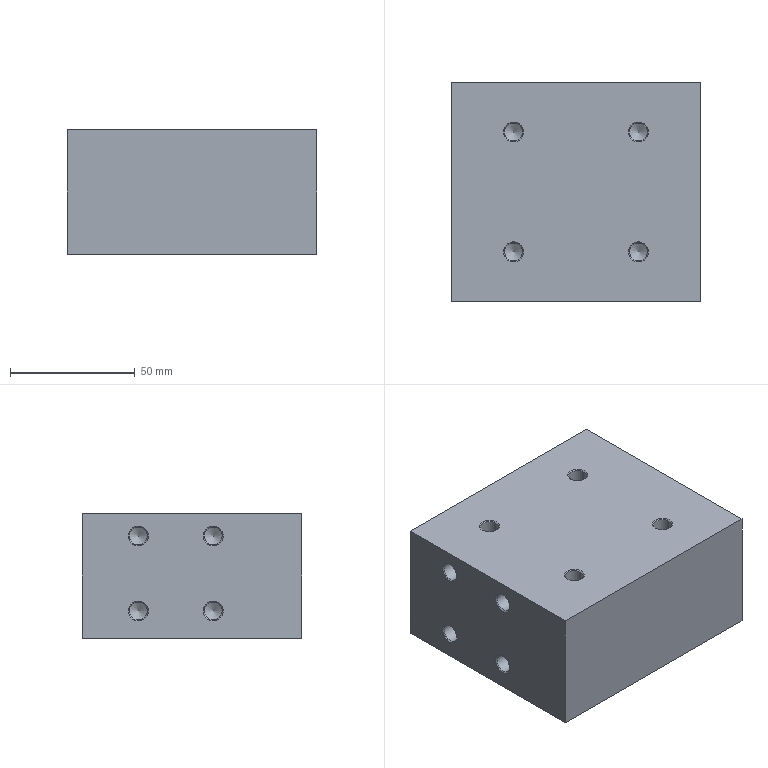Part | NX | features SIMPLE HOLE 8, SYMBOLIC_THREAD 8, DATUM_CSYS 4, SKETCH 3, HOLE PACKAGE 2, EXTRUDE 1 | 1 solid | 30 faces | box 100 x 88 x 50 mm | volume 433073 mm3 | cone 16 | cylinder 8 | plane 6 | commonest cylinder face diameters 7.2 x8
STEP:
#1=CARTESIAN_POINT('',(0.,69.5,41.));
#2=VERTEX_POINT('',#1);
#3=CARTESIAN_POINT('',(0.,65.5,41.));
#4=DIRECTION('',(1.,0.,0.));
#5=DIRECTION('',(0.,1.,0.));
#6=AXIS2_PLACEMENT_3D('',#3,#4,#5);
#7=CIRCLE('',#6,4.);
#8=EDGE_CURVE('',#2,#2,#7,.T.);
#9=ORIENTED_EDGE('',*,*,#8,.T.);
#10=EDGE_LOOP('',(#9));
#11=FACE_BOUND('',#10,.T.);
#12=CARTESIAN_POINT('',(0.,69.5,11.));
#13=VERTEX_POINT('',#12);
#14=CARTESIAN_POINT('',(0.,65.5,11.));
#15=DIRECTION('',(1.,0.,0.));
#16=DIRECTION('',(0.,1.,0.));
#17=AXIS2_PLACEMENT_3D('',#14,#15,#16);
#18=CIRCLE('',#17,4.);
#19=EDGE_CURVE('',#13,#13,#18,.T.);
#20=ORIENTED_EDGE('',*,*,#19,.T.);
#21=EDGE_LOOP('',(#20));
#22=FACE_BOUND('',#21,.T.);
#23=CARTESIAN_POINT('',(0.,39.5,41.));
#24=VERTEX_POINT('',#23);
#25=CARTESIAN_POINT('',(0.,35.5,41.));
#26=DIRECTION('',(1.,0.,0.));
#27=DIRECTION('',(0.,1.,0.));
#28=AXIS2_PLACEMENT_3D('',#25,#26,#27);
#29=CIRCLE('',#28,4.);
#30=EDGE_CURVE('',#24,#24,#29,.T.);
#31=ORIENTED_EDGE('',*,*,#30,.T.);
#32=EDGE_LOOP('',(#31));
#33=FACE_BOUND('',#32,.T.);
#34=CARTESIAN_POINT('',(0.,39.5,11.));
#35=VERTEX_POINT('',#34);
#36=CARTESIAN_POINT('',(0.,35.5,11.));
#37=DIRECTION('',(1.,0.,0.));
#38=DIRECTION('',(0.,1.,0.));
#39=AXIS2_PLACEMENT_3D('',#36,#37,#38);
#40=CIRCLE('',#39,4.);
#41=EDGE_CURVE('',#35,#35,#40,.T.);
#42=ORIENTED_EDGE('',*,*,#41,.T.);
#43=EDGE_LOOP('',(#42));
#44=FACE_BOUND('',#43,.T.);
#45=CARTESIAN_POINT('',(0.,88.,0.));
#46=VERTEX_POINT('',#45);
#47=CARTESIAN_POINT('',(0.,0.,0.));
#48=VERTEX_POINT('',#47);
#49=CARTESIAN_POINT('',(0.,88.,0.));
#50=DIRECTION('',(0.,-1.,0.));
#51=VECTOR('',#50,1000.);
#52=LINE('',#49,#51);
#53=EDGE_CURVE('',#46,#48,#52,.T.);
#54=ORIENTED_EDGE('',*,*,#53,.T.);
#55=CARTESIAN_POINT('',(0.,0.,50.));
#56=VERTEX_POINT('',#55);
#57=CARTESIAN_POINT('',(0.,0.,50.));
#58=DIRECTION('',(0.,0.,-1.));
#59=VECTOR('',#58,1000.);
#60=LINE('',#57,#59);
#61=EDGE_CURVE('',#56,#48,#60,.T.);
#62=ORIENTED_EDGE('',*,*,#61,.F.);
#63=CARTESIAN_POINT('',(0.,88.,50.));
#64=VERTEX_POINT('',#63);
#65=CARTESIAN_POINT('',(0.,88.,50.));
#66=DIRECTION('',(0.,-1.,0.));
#67=VECTOR('',#66,1000.);
#68=LINE('',#65,#67);
#69=EDGE_CURVE('',#64,#56,#68,.T.);
#70=ORIENTED_EDGE('',*,*,#69,.F.);
#71=CARTESIAN_POINT('',(0.,88.,50.));
#72=DIRECTION('',(0.,0.,-1.));
#73=VECTOR('',#72,1000.);
#74=LINE('',#71,#73);
#75=EDGE_CURVE('',#64,#46,#74,.T.);
#76=ORIENTED_EDGE('',*,*,#75,.T.);
#77=EDGE_LOOP('',(#54,#62,#70,#76));
#78=FACE_BOUND('',#77,.T.);
#79=CARTESIAN_POINT('',(0.,88.,50.));
#80=DIRECTION('',(1.,0.,0.));
#81=DIRECTION('',(0.,1.,0.));
#82=AXIS2_PLACEMENT_3D('',#79,#80,#81);
#83=PLANE('',#82);
#84=ADVANCED_FACE('',(#11,#22,#33,#44,#78),#83,.F.);
#85=CARTESIAN_POINT('',(100.,0.,0.));
#86=VERTEX_POINT('',#85);
#87=CARTESIAN_POINT('',(0.,0.,0.));
#88=DIRECTION('',(1.,0.,0.));
#89=VECTOR('',#88,1000.);
#90=LINE('',#87,#89);
#91=EDGE_CURVE('',#48,#86,#90,.T.);
#92=ORIENTED_EDGE('',*,*,#91,.T.);
#93=CARTESIAN_POINT('',(100.,0.,50.));
#94=VERTEX_POINT('',#93);
#95=CARTESIAN_POINT('',(100.,0.,50.));
#96=DIRECTION('',(0.,0.,-1.));
#97=VECTOR('',#96,1000.);
#98=LINE('',#95,#97);
#99=EDGE_CURVE('',#94,#86,#98,.T.);
#100=ORIENTED_EDGE('',*,*,#99,.F.);
#101=CARTESIAN_POINT('',(0.,0.,50.));
#102=DIRECTION('',(1.,0.,0.));
#103=VECTOR('',#102,1000.);
#104=LINE('',#101,#103);
#105=EDGE_CURVE('',#56,#94,#104,.T.);
#106=ORIENTED_EDGE('',*,*,#105,.F.);
#107=ORIENTED_EDGE('',*,*,#61,.T.);
#108=EDGE_LOOP('',(#92,#100,#106,#107));
#109=FACE_BOUND('',#108,.T.);
#110=CARTESIAN_POINT('',(0.,0.,50.));
#111=DIRECTION('',(0.,1.,0.));
#112=DIRECTION('',(0.,0.,1.));
#113=AXIS2_PLACEMENT_3D('',#110,#111,#112);
#114=PLANE('',#113);
#115=ADVANCED_FACE('',(#109),#114,.F.);
#116=CARTESIAN_POINT('',(100.,88.,0.));
#117=VERTEX_POINT('',#116);
#118=CARTESIAN_POINT('',(100.,0.,0.));
#119=DIRECTION('',(0.,1.,0.));
#120=VECTOR('',#119,1000.);
#121=LINE('',#118,#120);
#122=EDGE_CURVE('',#86,#117,#121,.T.);
#123=ORIENTED_EDGE('',*,*,#122,.T.);
#124=CARTESIAN_POINT('',(100.,88.,50.));
#125=VERTEX_POINT('',#124);
#126=CARTESIAN_POINT('',(100.,88.,50.));
#127=DIRECTION('',(0.,0.,-1.));
#128=VECTOR('',#127,1000.);
#129=LINE('',#126,#128);
#130=EDGE_CURVE('',#125,#117,#129,.T.);
#131=ORIENTED_EDGE('',*,*,#130,.F.);
#132=CARTESIAN_POINT('',(100.,0.,50.));
#133=DIRECTION('',(0.,1.,0.));
#134=VECTOR('',#133,1000.);
#135=LINE('',#132,#134);
#136=EDGE_CURVE('',#94,#125,#135,.T.);
#137=ORIENTED_EDGE('',*,*,#136,.F.);
#138=ORIENTED_EDGE('',*,*,#99,.T.);
#139=EDGE_LOOP('',(#123,#131,#137,#138));
#140=FACE_BOUND('',#139,.T.);
#141=CARTESIAN_POINT('',(100.,0.,50.));
#142=DIRECTION('',(-1.,0.,0.));
#143=DIRECTION('',(0.,-1.,0.));
#144=AXIS2_PLACEMENT_3D('',#141,#142,#143);
#145=PLANE('',#144);
#146=ADVANCED_FACE('',(#140),#145,.F.);
#147=CARTESIAN_POINT('',(100.,88.,0.));
#148=DIRECTION('',(-1.,0.,0.));
#149=VECTOR('',#148,1000.);
#150=LINE('',#147,#149);
#151=EDGE_CURVE('',#117,#46,#150,.T.);
#152=ORIENTED_EDGE('',*,*,#151,.T.);
#153=ORIENTED_EDGE('',*,*,#75,.F.);
#154=CARTESIAN_POINT('',(100.,88.,50.));
#155=DIRECTION('',(-1.,0.,0.));
#156=VECTOR('',#155,1000.);
#157=LINE('',#154,#156);
#158=EDGE_CURVE('',#125,#64,#157,.T.);
#159=ORIENTED_EDGE('',*,*,#158,.F.);
#160=ORIENTED_EDGE('',*,*,#130,.T.);
#161=EDGE_LOOP('',(#152,#153,#159,#160));
#162=FACE_BOUND('',#161,.T.);
#163=CARTESIAN_POINT('',(100.,88.,50.));
#164=DIRECTION('',(0.,-1.,0.));
#165=DIRECTION('',(1.,0.,0.));
#166=AXIS2_PLACEMENT_3D('',#163,#164,#165);
#167=PLANE('',#166);
#168=ADVANCED_FACE('',(#162),#167,.F.);
#169=CARTESIAN_POINT('',(79.,68.,50.));
#170=VERTEX_POINT('',#169);
#171=CARTESIAN_POINT('',(75.,68.,50.));
#172=DIRECTION('',(0.,0.,1.));
#173=DIRECTION('',(1.,0.,0.));
#174=AXIS2_PLACEMENT_3D('',#171,#172,#173);
#175=CIRCLE('',#174,4.);
#176=EDGE_CURVE('',#170,#170,#175,.F.);
#177=ORIENTED_EDGE('',*,*,#176,.T.);
#178=EDGE_LOOP('',(#177));
#179=FACE_BOUND('',#178,.T.);
#180=CARTESIAN_POINT('',(29.,68.,50.));
#181=VERTEX_POINT('',#180);
#182=CARTESIAN_POINT('',(25.,68.,50.));
#183=DIRECTION('',(0.,0.,1.));
#184=DIRECTION('',(1.,0.,0.));
#185=AXIS2_PLACEMENT_3D('',#182,#183,#184);
#186=CIRCLE('',#185,4.);
#187=EDGE_CURVE('',#181,#181,#186,.F.);
#188=ORIENTED_EDGE('',*,*,#187,.T.);
#189=EDGE_LOOP('',(#188));
#190=FACE_BOUND('',#189,.T.);
#191=CARTESIAN_POINT('',(29.,20.,50.));
#192=VERTEX_POINT('',#191);
#193=CARTESIAN_POINT('',(25.,20.,50.));
#194=DIRECTION('',(0.,0.,1.));
#195=DIRECTION('',(1.,0.,0.));
#196=AXIS2_PLACEMENT_3D('',#193,#194,#195);
#197=CIRCLE('',#196,4.);
#198=EDGE_CURVE('',#192,#192,#197,.F.);
#199=ORIENTED_EDGE('',*,*,#198,.T.);
#200=EDGE_LOOP('',(#199));
#201=FACE_BOUND('',#200,.T.);
#202=CARTESIAN_POINT('',(79.,20.,50.));
#203=VERTEX_POINT('',#202);
#204=CARTESIAN_POINT('',(75.,20.,50.));
#205=DIRECTION('',(0.,0.,1.));
#206=DIRECTION('',(1.,0.,0.));
#207=AXIS2_PLACEMENT_3D('',#204,#205,#206);
#208=CIRCLE('',#207,4.);
#209=EDGE_CURVE('',#203,#203,#208,.F.);
#210=ORIENTED_EDGE('',*,*,#209,.T.);
#211=EDGE_LOOP('',(#210));
#212=FACE_BOUND('',#211,.T.);
#213=ORIENTED_EDGE('',*,*,#69,.T.);
#214=ORIENTED_EDGE('',*,*,#105,.T.);
#215=ORIENTED_EDGE('',*,*,#136,.T.);
#216=ORIENTED_EDGE('',*,*,#158,.T.);
#217=EDGE_LOOP('',(#213,#214,#215,#216));
#218=FACE_BOUND('',#217,.T.);
#219=CARTESIAN_POINT('',(0.,0.,50.));
#220=DIRECTION('',(0.,0.,1.));
#221=DIRECTION('',(1.,0.,0.));
#222=AXIS2_PLACEMENT_3D('',#219,#220,#221);
#223=PLANE('',#222);
#224=ADVANCED_FACE('',(#179,#190,#201,#212,#218),#223,.T.);
#225=ORIENTED_EDGE('',*,*,#53,.F.);
#226=ORIENTED_EDGE('',*,*,#151,.F.);
#227=ORIENTED_EDGE('',*,*,#122,.F.);
#228=ORIENTED_EDGE('',*,*,#91,.F.);
#229=EDGE_LOOP('',(#225,#226,#227,#228));
#230=FACE_BOUND('',#229,.T.);
#231=CARTESIAN_POINT('',(0.,0.,0.));
#232=DIRECTION('',(0.,0.,1.));
#233=DIRECTION('',(1.,0.,0.));
#234=AXIS2_PLACEMENT_3D('',#231,#232,#233);
#235=PLANE('',#234);
#236=ADVANCED_FACE('',(#230),#235,.F.);
#237=CARTESIAN_POINT('',(18.,39.1,11.));
#238=VERTEX_POINT('',#237);
#239=CARTESIAN_POINT('',(18.,35.5,11.));
#240=DIRECTION('',(1.,0.,0.));
#241=DIRECTION('',(0.,1.,0.));
#242=AXIS2_PLACEMENT_3D('',#239,#240,#241);
#243=CIRCLE('',#242,3.6);
#244=EDGE_CURVE('',#238,#238,#243,.F.);
#245=ORIENTED_EDGE('',*,*,#244,.T.);
#246=EDGE_LOOP('',(#245));
#247=FACE_BOUND('',#246,.T.);
#248=CARTESIAN_POINT('',(20.163,35.5,11.));
#249=VERTEX_POINT('',#248);
#250=VERTEX_LOOP('',#249);
#251=FACE_BOUND('',#250,.T.);
#252=CARTESIAN_POINT('',(18.,35.5,11.));
#253=DIRECTION('',(-1.,0.,0.));
#254=DIRECTION('',(0.,-1.,0.));
#255=AXIS2_PLACEMENT_3D('',#252,#253,#254);
#256=CONICAL_SURFACE('',#255,3.6,1.03);
#257=ADVANCED_FACE('',(#247,#251),#256,.F.);
#258=CARTESIAN_POINT('',(0.4,35.5,7.4));
#259=VERTEX_POINT('',#258);
#260=CARTESIAN_POINT('',(0.4,35.5,11.));
#261=DIRECTION('',(1.,0.,0.));
#262=DIRECTION('',(0.,0.,-1.));
#263=AXIS2_PLACEMENT_3D('',#260,#261,#262);
#264=CIRCLE('',#263,3.6);
#265=EDGE_CURVE('',#259,#259,#264,.F.);
#266=ORIENTED_EDGE('',*,*,#265,.T.);
#267=EDGE_LOOP('',(#266));
#268=FACE_BOUND('',#267,.T.);
#269=ORIENTED_EDGE('',*,*,#244,.F.);
#270=EDGE_LOOP('',(#269));
#271=FACE_BOUND('',#270,.T.);
#272=CARTESIAN_POINT('',(0.,35.5,11.));
#273=DIRECTION('',(1.,0.,0.));
#274=DIRECTION('',(0.,1.,0.));
#275=AXIS2_PLACEMENT_3D('',#272,#273,#274);
#276=CYLINDRICAL_SURFACE('',#275,3.6);
#277=ADVANCED_FACE('',(#268,#271),#276,.F.);
#278=ORIENTED_EDGE('',*,*,#265,.F.);
#279=EDGE_LOOP('',(#278));
#280=FACE_BOUND('',#279,.T.);
#281=ORIENTED_EDGE('',*,*,#41,.F.);
#282=EDGE_LOOP('',(#281));
#283=FACE_BOUND('',#282,.T.);
#284=CARTESIAN_POINT('',(0.,35.5,11.));
#285=DIRECTION('',(-1.,0.,0.));
#286=DIRECTION('',(0.,0.,1.));
#287=AXIS2_PLACEMENT_3D('',#284,#285,#286);
#288=CONICAL_SURFACE('',#287,4.,0.7854);
#289=ADVANCED_FACE('',(#280,#283),#288,.F.);
#290=CARTESIAN_POINT('',(18.,39.1,41.));
#291=VERTEX_POINT('',#290);
#292=CARTESIAN_POINT('',(18.,35.5,41.));
#293=DIRECTION('',(1.,0.,0.));
#294=DIRECTION('',(0.,1.,0.));
#295=AXIS2_PLACEMENT_3D('',#292,#293,#294);
#296=CIRCLE('',#295,3.6);
#297=EDGE_CURVE('',#291,#291,#296,.F.);
#298=ORIENTED_EDGE('',*,*,#297,.T.);
#299=EDGE_LOOP('',(#298));
#300=FACE_BOUND('',#299,.T.);
#301=CARTESIAN_POINT('',(20.163,35.5,41.));
#302=VERTEX_POINT('',#301);
#303=VERTEX_LOOP('',#302);
#304=FACE_BOUND('',#303,.T.);
#305=CARTESIAN_POINT('',(18.,35.5,41.));
#306=DIRECTION('',(-1.,0.,0.));
#307=DIRECTION('',(0.,-1.,0.));
#308=AXIS2_PLACEMENT_3D('',#305,#306,#307);
#309=CONICAL_SURFACE('',#308,3.6,1.03);
#310=ADVANCED_FACE('',(#300,#304),#309,.F.);
#311=CARTESIAN_POINT('',(0.4,35.5,37.4));
#312=VERTEX_POINT('',#311);
#313=CARTESIAN_POINT('',(0.4,35.5,41.));
#314=DIRECTION('',(1.,0.,0.));
#315=DIRECTION('',(0.,0.,-1.));
#316=AXIS2_PLACEMENT_3D('',#313,#314,#315);
#317=CIRCLE('',#316,3.6);
#318=EDGE_CURVE('',#312,#312,#317,.F.);
#319=ORIENTED_EDGE('',*,*,#318,.T.);
#320=EDGE_LOOP('',(#319));
#321=FACE_BOUND('',#320,.T.);
#322=ORIENTED_EDGE('',*,*,#297,.F.);
#323=EDGE_LOOP('',(#322));
#324=FACE_BOUND('',#323,.T.);
#325=CARTESIAN_POINT('',(0.,35.5,41.));
#326=DIRECTION('',(1.,0.,0.));
#327=DIRECTION('',(0.,1.,0.));
#328=AXIS2_PLACEMENT_3D('',#325,#326,#327);
#329=CYLINDRICAL_SURFACE('',#328,3.6);
#330=ADVANCED_FACE('',(#321,#324),#329,.F.);
#331=ORIENTED_EDGE('',*,*,#318,.F.);
#332=EDGE_LOOP('',(#331));
#333=FACE_BOUND('',#332,.T.);
#334=ORIENTED_EDGE('',*,*,#30,.F.);
#335=EDGE_LOOP('',(#334));
#336=FACE_BOUND('',#335,.T.);
#337=CARTESIAN_POINT('',(0.,35.5,41.));
#338=DIRECTION('',(-1.,0.,0.));
#339=DIRECTION('',(0.,0.,1.));
#340=AXIS2_PLACEMENT_3D('',#337,#338,#339);
#341=CONICAL_SURFACE('',#340,4.,0.7854);
#342=ADVANCED_FACE('',(#333,#336),#341,.F.);
#343=CARTESIAN_POINT('',(18.,69.1,11.));
#344=VERTEX_POINT('',#343);
#345=CARTESIAN_POINT('',(18.,65.5,11.));
#346=DIRECTION('',(1.,0.,0.));
#347=DIRECTION('',(0.,1.,0.));
#348=AXIS2_PLACEMENT_3D('',#345,#346,#347);
#349=CIRCLE('',#348,3.6);
#350=EDGE_CURVE('',#344,#344,#349,.F.);
#351=ORIENTED_EDGE('',*,*,#350,.T.);
#352=EDGE_LOOP('',(#351));
#353=FACE_BOUND('',#352,.T.);
#354=CARTESIAN_POINT('',(20.163,65.5,11.));
#355=VERTEX_POINT('',#354);
#356=VERTEX_LOOP('',#355);
#357=FACE_BOUND('',#356,.T.);
#358=CARTESIAN_POINT('',(18.,65.5,11.));
#359=DIRECTION('',(-1.,0.,0.));
#360=DIRECTION('',(0.,-1.,0.));
#361=AXIS2_PLACEMENT_3D('',#358,#359,#360);
#362=CONICAL_SURFACE('',#361,3.6,1.03);
#363=ADVANCED_FACE('',(#353,#357),#362,.F.);
#364=CARTESIAN_POINT('',(0.4,65.5,7.4));
#365=VERTEX_POINT('',#364);
#366=CARTESIAN_POINT('',(0.4,65.5,11.));
#367=DIRECTION('',(1.,0.,0.));
#368=DIRECTION('',(0.,0.,-1.));
#369=AXIS2_PLACEMENT_3D('',#366,#367,#368);
#370=CIRCLE('',#369,3.6);
#371=EDGE_CURVE('',#365,#365,#370,.F.);
#372=ORIENTED_EDGE('',*,*,#371,.T.);
#373=EDGE_LOOP('',(#372));
#374=FACE_BOUND('',#373,.T.);
#375=ORIENTED_EDGE('',*,*,#350,.F.);
#376=EDGE_LOOP('',(#375));
#377=FACE_BOUND('',#376,.T.);
#378=CARTESIAN_POINT('',(0.,65.5,11.));
#379=DIRECTION('',(1.,0.,0.));
#380=DIRECTION('',(0.,1.,0.));
#381=AXIS2_PLACEMENT_3D('',#378,#379,#380);
#382=CYLINDRICAL_SURFACE('',#381,3.6);
#383=ADVANCED_FACE('',(#374,#377),#382,.F.);
#384=ORIENTED_EDGE('',*,*,#371,.F.);
#385=EDGE_LOOP('',(#384));
#386=FACE_BOUND('',#385,.T.);
#387=ORIENTED_EDGE('',*,*,#19,.F.);
#388=EDGE_LOOP('',(#387));
#389=FACE_BOUND('',#388,.T.);
#390=CARTESIAN_POINT('',(0.,65.5,11.));
#391=DIRECTION('',(-1.,0.,0.));
#392=DIRECTION('',(0.,0.,1.));
#393=AXIS2_PLACEMENT_3D('',#390,#391,#392);
#394=CONICAL_SURFACE('',#393,4.,0.7854);
#395=ADVANCED_FACE('',(#386,#389),#394,.F.);
#396=CARTESIAN_POINT('',(18.,69.1,41.));
#397=VERTEX_POINT('',#396);
#398=CARTESIAN_POINT('',(18.,65.5,41.));
#399=DIRECTION('',(1.,0.,0.));
#400=DIRECTION('',(0.,1.,0.));
#401=AXIS2_PLACEMENT_3D('',#398,#399,#400);
#402=CIRCLE('',#401,3.6);
#403=EDGE_CURVE('',#397,#397,#402,.F.);
#404=ORIENTED_EDGE('',*,*,#403,.T.);
#405=EDGE_LOOP('',(#404));
#406=FACE_BOUND('',#405,.T.);
#407=CARTESIAN_POINT('',(20.163,65.5,41.));
#408=VERTEX_POINT('',#407);
#409=VERTEX_LOOP('',#408);
#410=FACE_BOUND('',#409,.T.);
#411=CARTESIAN_POINT('',(18.,65.5,41.));
#412=DIRECTION('',(-1.,0.,0.));
#413=DIRECTION('',(0.,-1.,0.));
#414=AXIS2_PLACEMENT_3D('',#411,#412,#413);
#415=CONICAL_SURFACE('',#414,3.6,1.03);
#416=ADVANCED_FACE('',(#406,#410),#415,.F.);
#417=CARTESIAN_POINT('',(0.4,65.5,37.4));
#418=VERTEX_POINT('',#417);
#419=CARTESIAN_POINT('',(0.4,65.5,41.));
#420=DIRECTION('',(1.,0.,0.));
#421=DIRECTION('',(0.,0.,-1.));
#422=AXIS2_PLACEMENT_3D('',#419,#420,#421);
#423=CIRCLE('',#422,3.6);
#424=EDGE_CURVE('',#418,#418,#423,.F.);
#425=ORIENTED_EDGE('',*,*,#424,.T.);
#426=EDGE_LOOP('',(#425));
#427=FACE_BOUND('',#426,.T.);
#428=ORIENTED_EDGE('',*,*,#403,.F.);
#429=EDGE_LOOP('',(#428));
#430=FACE_BOUND('',#429,.T.);
#431=CARTESIAN_POINT('',(0.,65.5,41.));
#432=DIRECTION('',(1.,0.,0.));
#433=DIRECTION('',(0.,1.,0.));
#434=AXIS2_PLACEMENT_3D('',#431,#432,#433);
#435=CYLINDRICAL_SURFACE('',#434,3.6);
#436=ADVANCED_FACE('',(#427,#430),#435,.F.);
#437=ORIENTED_EDGE('',*,*,#424,.F.);
#438=EDGE_LOOP('',(#437));
#439=FACE_BOUND('',#438,.T.);
#440=ORIENTED_EDGE('',*,*,#8,.F.);
#441=EDGE_LOOP('',(#440));
#442=FACE_BOUND('',#441,.T.);
#443=CARTESIAN_POINT('',(0.,65.5,41.));
#444=DIRECTION('',(-1.,0.,0.));
#445=DIRECTION('',(0.,0.,1.));
#446=AXIS2_PLACEMENT_3D('',#443,#444,#445);
#447=CONICAL_SURFACE('',#446,4.,0.7854);
#448=ADVANCED_FACE('',(#439,#442),#447,.F.);
#449=CARTESIAN_POINT('',(71.4,20.,27.));
#450=VERTEX_POINT('',#449);
#451=CARTESIAN_POINT('',(75.,20.,27.));
#452=DIRECTION('',(0.,0.,-1.));
#453=DIRECTION('',(-1.,0.,0.));
#454=AXIS2_PLACEMENT_3D('',#451,#452,#453);
#455=CIRCLE('',#454,3.6);
#456=EDGE_CURVE('',#450,#450,#455,.F.);
#457=ORIENTED_EDGE('',*,*,#456,.T.);
#458=EDGE_LOOP('',(#457));
#459=FACE_BOUND('',#458,.T.);
#460=CARTESIAN_POINT('',(75.,20.,24.837));
#461=VERTEX_POINT('',#460);
#462=VERTEX_LOOP('',#461);
#463=FACE_BOUND('',#462,.T.);
#464=CARTESIAN_POINT('',(75.,20.,27.));
#465=DIRECTION('',(0.,0.,1.));
#466=DIRECTION('',(1.,0.,0.));
#467=AXIS2_PLACEMENT_3D('',#464,#465,#466);
#468=CONICAL_SURFACE('',#467,3.6,1.03);
#469=ADVANCED_FACE('',(#459,#463),#468,.F.);
#470=CARTESIAN_POINT('',(78.6,20.,49.6));
#471=VERTEX_POINT('',#470);
#472=CARTESIAN_POINT('',(75.,20.,49.6));
#473=DIRECTION('',(0.,0.,1.));
#474=DIRECTION('',(1.,0.,0.));
#475=AXIS2_PLACEMENT_3D('',#472,#473,#474);
#476=CIRCLE('',#475,3.6);
#477=EDGE_CURVE('',#471,#471,#476,.T.);
#478=ORIENTED_EDGE('',*,*,#477,.T.);
#479=EDGE_LOOP('',(#478));
#480=FACE_BOUND('',#479,.T.);
#481=ORIENTED_EDGE('',*,*,#456,.F.);
#482=EDGE_LOOP('',(#481));
#483=FACE_BOUND('',#482,.T.);
#484=CARTESIAN_POINT('',(75.,20.,50.));
#485=DIRECTION('',(0.,0.,-1.));
#486=DIRECTION('',(-1.,0.,0.));
#487=AXIS2_PLACEMENT_3D('',#484,#485,#486);
#488=CYLINDRICAL_SURFACE('',#487,3.6);
#489=ADVANCED_FACE('',(#480,#483),#488,.F.);
#490=ORIENTED_EDGE('',*,*,#477,.F.);
#491=EDGE_LOOP('',(#490));
#492=FACE_BOUND('',#491,.T.);
#493=ORIENTED_EDGE('',*,*,#209,.F.);
#494=EDGE_LOOP('',(#493));
#495=FACE_BOUND('',#494,.T.);
#496=CARTESIAN_POINT('',(75.,20.,50.));
#497=DIRECTION('',(0.,0.,1.));
#498=DIRECTION('',(1.,0.,0.));
#499=AXIS2_PLACEMENT_3D('',#496,#497,#498);
#500=CONICAL_SURFACE('',#499,4.,0.7854);
#501=ADVANCED_FACE('',(#492,#495),#500,.F.);
#502=CARTESIAN_POINT('',(21.4,20.,27.));
#503=VERTEX_POINT('',#502);
#504=CARTESIAN_POINT('',(25.,20.,27.));
#505=DIRECTION('',(0.,0.,-1.));
#506=DIRECTION('',(-1.,0.,0.));
#507=AXIS2_PLACEMENT_3D('',#504,#505,#506);
#508=CIRCLE('',#507,3.6);
#509=EDGE_CURVE('',#503,#503,#508,.F.);
#510=ORIENTED_EDGE('',*,*,#509,.T.);
#511=EDGE_LOOP('',(#510));
#512=FACE_BOUND('',#511,.T.);
#513=CARTESIAN_POINT('',(25.,20.,24.837));
#514=VERTEX_POINT('',#513);
#515=VERTEX_LOOP('',#514);
#516=FACE_BOUND('',#515,.T.);
#517=CARTESIAN_POINT('',(25.,20.,27.));
#518=DIRECTION('',(0.,0.,1.));
#519=DIRECTION('',(1.,0.,0.));
#520=AXIS2_PLACEMENT_3D('',#517,#518,#519);
#521=CONICAL_SURFACE('',#520,3.6,1.03);
#522=ADVANCED_FACE('',(#512,#516),#521,.F.);
#523=CARTESIAN_POINT('',(28.6,20.,49.6));
#524=VERTEX_POINT('',#523);
#525=CARTESIAN_POINT('',(25.,20.,49.6));
#526=DIRECTION('',(0.,0.,1.));
#527=DIRECTION('',(1.,0.,0.));
#528=AXIS2_PLACEMENT_3D('',#525,#526,#527);
#529=CIRCLE('',#528,3.6);
#530=EDGE_CURVE('',#524,#524,#529,.T.);
#531=ORIENTED_EDGE('',*,*,#530,.T.);
#532=EDGE_LOOP('',(#531));
#533=FACE_BOUND('',#532,.T.);
#534=ORIENTED_EDGE('',*,*,#509,.F.);
#535=EDGE_LOOP('',(#534));
#536=FACE_BOUND('',#535,.T.);
#537=CARTESIAN_POINT('',(25.,20.,50.));
#538=DIRECTION('',(0.,0.,-1.));
#539=DIRECTION('',(-1.,0.,0.));
#540=AXIS2_PLACEMENT_3D('',#537,#538,#539);
#541=CYLINDRICAL_SURFACE('',#540,3.6);
#542=ADVANCED_FACE('',(#533,#536),#541,.F.);
#543=ORIENTED_EDGE('',*,*,#530,.F.);
#544=EDGE_LOOP('',(#543));
#545=FACE_BOUND('',#544,.T.);
#546=ORIENTED_EDGE('',*,*,#198,.F.);
#547=EDGE_LOOP('',(#546));
#548=FACE_BOUND('',#547,.T.);
#549=CARTESIAN_POINT('',(25.,20.,50.));
#550=DIRECTION('',(0.,0.,1.));
#551=DIRECTION('',(1.,0.,0.));
#552=AXIS2_PLACEMENT_3D('',#549,#550,#551);
#553=CONICAL_SURFACE('',#552,4.,0.7854);
#554=ADVANCED_FACE('',(#545,#548),#553,.F.);
#555=CARTESIAN_POINT('',(21.4,68.,27.));
#556=VERTEX_POINT('',#555);
#557=CARTESIAN_POINT('',(25.,68.,27.));
#558=DIRECTION('',(0.,0.,-1.));
#559=DIRECTION('',(-1.,0.,0.));
#560=AXIS2_PLACEMENT_3D('',#557,#558,#559);
#561=CIRCLE('',#560,3.6);
#562=EDGE_CURVE('',#556,#556,#561,.F.);
#563=ORIENTED_EDGE('',*,*,#562,.T.);
#564=EDGE_LOOP('',(#563));
#565=FACE_BOUND('',#564,.T.);
#566=CARTESIAN_POINT('',(25.,68.,24.837));
#567=VERTEX_POINT('',#566);
#568=VERTEX_LOOP('',#567);
#569=FACE_BOUND('',#568,.T.);
#570=CARTESIAN_POINT('',(25.,68.,27.));
#571=DIRECTION('',(0.,0.,1.));
#572=DIRECTION('',(1.,0.,0.));
#573=AXIS2_PLACEMENT_3D('',#570,#571,#572);
#574=CONICAL_SURFACE('',#573,3.6,1.03);
#575=ADVANCED_FACE('',(#565,#569),#574,.F.);
#576=CARTESIAN_POINT('',(28.6,68.,49.6));
#577=VERTEX_POINT('',#576);
#578=CARTESIAN_POINT('',(25.,68.,49.6));
#579=DIRECTION('',(0.,0.,1.));
#580=DIRECTION('',(1.,0.,0.));
#581=AXIS2_PLACEMENT_3D('',#578,#579,#580);
#582=CIRCLE('',#581,3.6);
#583=EDGE_CURVE('',#577,#577,#582,.T.);
#584=ORIENTED_EDGE('',*,*,#583,.T.);
#585=EDGE_LOOP('',(#584));
#586=FACE_BOUND('',#585,.T.);
#587=ORIENTED_EDGE('',*,*,#562,.F.);
#588=EDGE_LOOP('',(#587));
#589=FACE_BOUND('',#588,.T.);
#590=CARTESIAN_POINT('',(25.,68.,50.));
#591=DIRECTION('',(0.,0.,-1.));
#592=DIRECTION('',(-1.,0.,0.));
#593=AXIS2_PLACEMENT_3D('',#590,#591,#592);
#594=CYLINDRICAL_SURFACE('',#593,3.6);
#595=ADVANCED_FACE('',(#586,#589),#594,.F.);
#596=ORIENTED_EDGE('',*,*,#583,.F.);
#597=EDGE_LOOP('',(#596));
#598=FACE_BOUND('',#597,.T.);
#599=ORIENTED_EDGE('',*,*,#187,.F.);
#600=EDGE_LOOP('',(#599));
#601=FACE_BOUND('',#600,.T.);
#602=CARTESIAN_POINT('',(25.,68.,50.));
#603=DIRECTION('',(0.,0.,1.));
#604=DIRECTION('',(1.,0.,0.));
#605=AXIS2_PLACEMENT_3D('',#602,#603,#604);
#606=CONICAL_SURFACE('',#605,4.,0.7854);
#607=ADVANCED_FACE('',(#598,#601),#606,.F.);
#608=CARTESIAN_POINT('',(71.4,68.,27.));
#609=VERTEX_POINT('',#608);
#610=CARTESIAN_POINT('',(75.,68.,27.));
#611=DIRECTION('',(0.,0.,-1.));
#612=DIRECTION('',(-1.,0.,0.));
#613=AXIS2_PLACEMENT_3D('',#610,#611,#612);
#614=CIRCLE('',#613,3.6);
#615=EDGE_CURVE('',#609,#609,#614,.F.);
#616=ORIENTED_EDGE('',*,*,#615,.T.);
#617=EDGE_LOOP('',(#616));
#618=FACE_BOUND('',#617,.T.);
#619=CARTESIAN_POINT('',(75.,68.,24.837));
#620=VERTEX_POINT('',#619);
#621=VERTEX_LOOP('',#620);
#622=FACE_BOUND('',#621,.T.);
#623=CARTESIAN_POINT('',(75.,68.,27.));
#624=DIRECTION('',(0.,0.,1.));
#625=DIRECTION('',(1.,0.,0.));
#626=AXIS2_PLACEMENT_3D('',#623,#624,#625);
#627=CONICAL_SURFACE('',#626,3.6,1.03);
#628=ADVANCED_FACE('',(#618,#622),#627,.F.);
#629=CARTESIAN_POINT('',(78.6,68.,49.6));
#630=VERTEX_POINT('',#629);
#631=CARTESIAN_POINT('',(75.,68.,49.6));
#632=DIRECTION('',(0.,0.,1.));
#633=DIRECTION('',(1.,0.,0.));
#634=AXIS2_PLACEMENT_3D('',#631,#632,#633);
#635=CIRCLE('',#634,3.6);
#636=EDGE_CURVE('',#630,#630,#635,.T.);
#637=ORIENTED_EDGE('',*,*,#636,.T.);
#638=EDGE_LOOP('',(#637));
#639=FACE_BOUND('',#638,.T.);
#640=ORIENTED_EDGE('',*,*,#615,.F.);
#641=EDGE_LOOP('',(#640));
#642=FACE_BOUND('',#641,.T.);
#643=CARTESIAN_POINT('',(75.,68.,50.));
#644=DIRECTION('',(0.,0.,-1.));
#645=DIRECTION('',(-1.,0.,0.));
#646=AXIS2_PLACEMENT_3D('',#643,#644,#645);
#647=CYLINDRICAL_SURFACE('',#646,3.6);
#648=ADVANCED_FACE('',(#639,#642),#647,.F.);
#649=ORIENTED_EDGE('',*,*,#636,.F.);
#650=EDGE_LOOP('',(#649));
#651=FACE_BOUND('',#650,.T.);
#652=ORIENTED_EDGE('',*,*,#176,.F.);
#653=EDGE_LOOP('',(#652));
#654=FACE_BOUND('',#653,.T.);
#655=CARTESIAN_POINT('',(75.,68.,50.));
#656=DIRECTION('',(0.,0.,1.));
#657=DIRECTION('',(1.,0.,0.));
#658=AXIS2_PLACEMENT_3D('',#655,#656,#657);
#659=CONICAL_SURFACE('',#658,4.,0.7854);
#660=ADVANCED_FACE('',(#651,#654),#659,.F.);
#661=CLOSED_SHELL('',(#84,#115,#146,#168,#224,#236,#257,#277,#289,#310,#330,#342,#363,#383,#395,#416,#436,#448,#469,#489,#501,#522,#542,#554,#575,#595,#607,#628,#648,#660));
#662=MANIFOLD_SOLID_BREP('',#661);
#663=(LENGTH_UNIT()NAMED_UNIT(*)SI_UNIT(.MILLI.,.METRE.));
#664=UNCERTAINTY_MEASURE_WITH_UNIT(LENGTH_MEASURE(0.00001),#663,'','');
#665=(NAMED_UNIT(*)PLANE_ANGLE_UNIT()SI_UNIT($,.RADIAN.));
#666=(NAMED_UNIT(*)SI_UNIT($,.STERADIAN.)SOLID_ANGLE_UNIT());
#667=(GEOMETRIC_REPRESENTATION_CONTEXT(3)GLOBAL_UNCERTAINTY_ASSIGNED_CONTEXT((#664))GLOBAL_UNIT_ASSIGNED_CONTEXT((#663,#665,#666))REPRESENTATION_CONTEXT('',''));
#668=ADVANCED_BREP_SHAPE_REPRESENTATION('',(#662),#667);